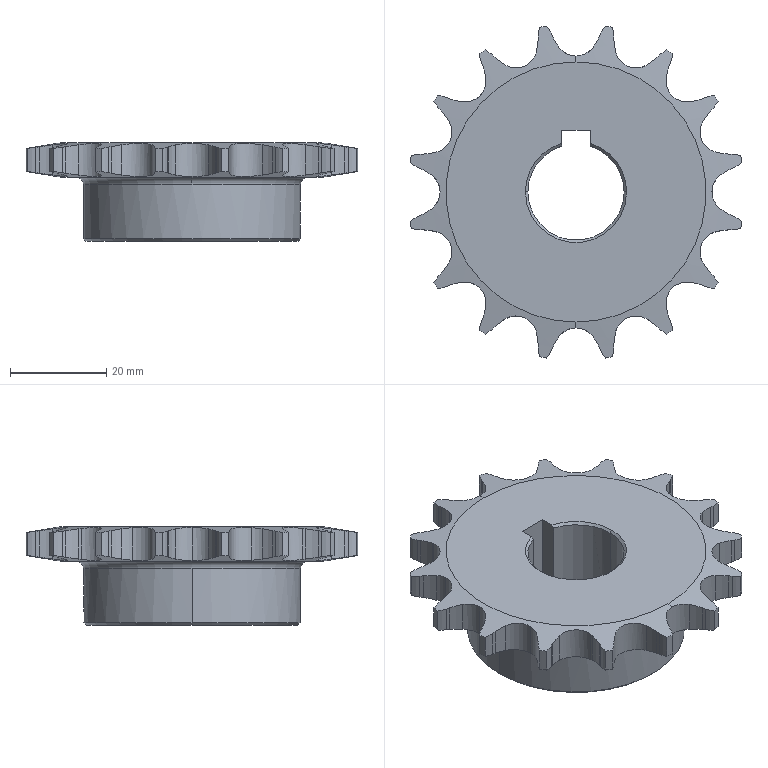Part | STEP file | 1 solid | 162 faces | box 68.92 x 68.92 x 20.5 mm | volume 34820 mm3 | cylinder 110 | plane 38 | cone 12 | torus 2 | commonest cylinder face diameters 12.473 x32 22.269 x32 8.653 x21 70 x16 4.2 x4 20 x3